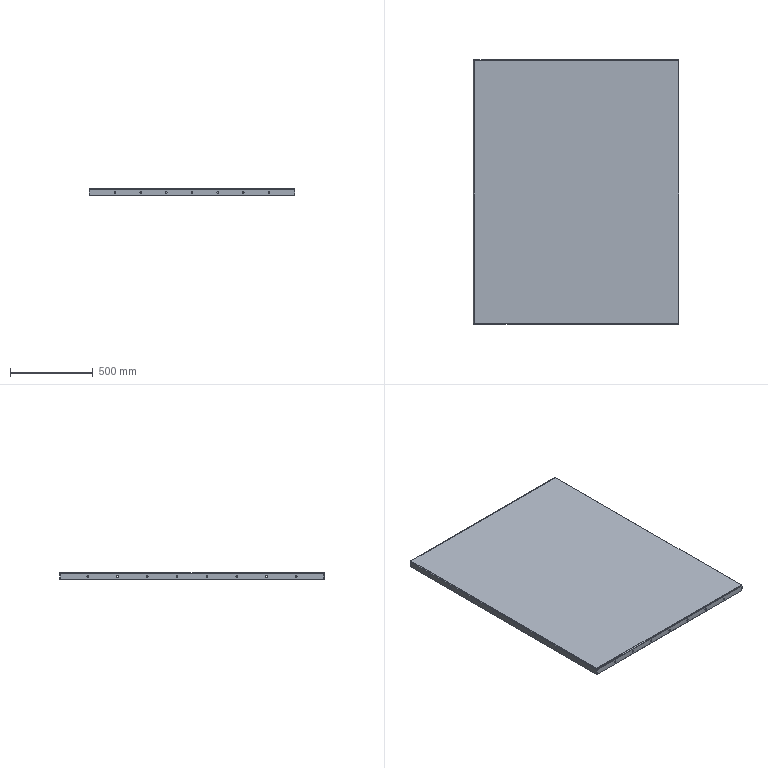Part | SolidWorks | features ICE 2, CornerFeat 1, EdgeFlange 1, FlatPattern 1, SMBaseFlange 1, SheetMetal 1 | 1 solid | 60 faces | box 1240 x 1600 x 40 mm | volume 6376482 mm3 | cylinder 36 | plane 20 | spline 4 | commonest cylinder face diameters 10 x30 6 x3 12 x3